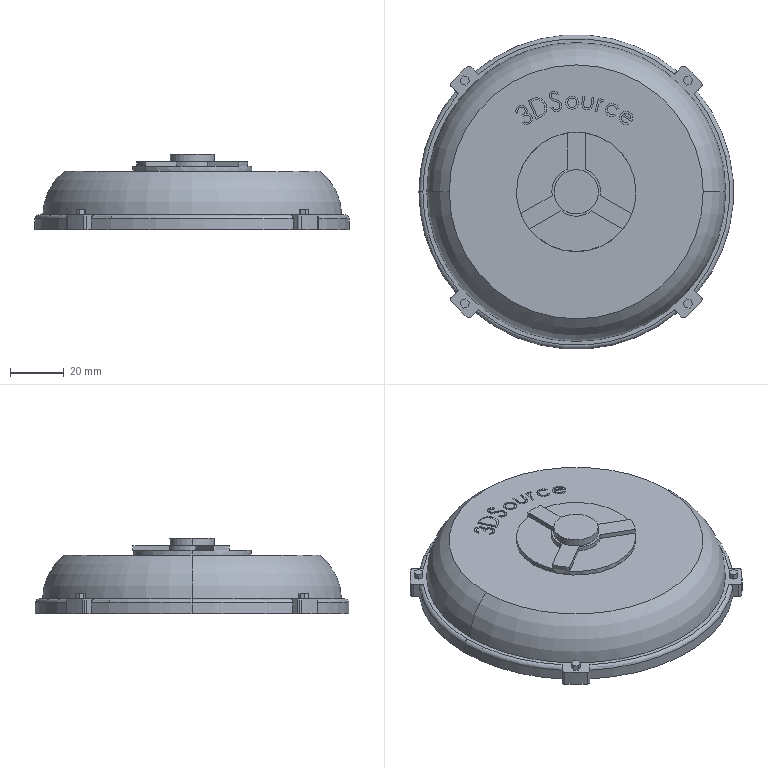Part | NX | features BREP 1 | 1 solid | 164 faces | box 117 x 117 x 28 mm | volume 208351 mm3 | plane 94 | cylinder 63 | torus 7 | commonest cylinder face diameters 2.08 x10 2.791 x8 3.459 x6 4.855 x6 4.157 x5 117 x5